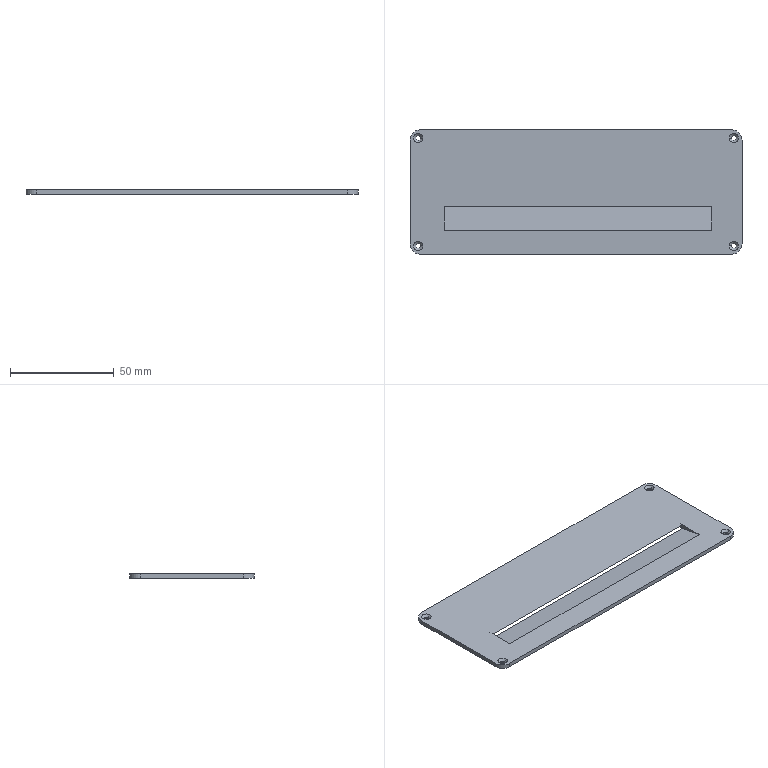Part | SolidWorks | features ICE 2, Extrusion 1, Fillet 1, HoleWzd 1 | 1 solid | 30 faces | box 160 x 60 x 2 mm | volume 16130 mm3 | cylinder 12 | plane 10 | cone 8 | commonest cylinder face diameters 2.4 x8 10 x4
STEP:
#1=CARTESIAN_POINT('',(-77.2,26.,0.95));
#2=VERTEX_POINT('',#1);
#3=CARTESIAN_POINT('',(-74.8,26.,0.95));
#4=VERTEX_POINT('',#3);
#5=CARTESIAN_POINT('',(-76.,26.,0.95));
#6=DIRECTION('',(0.,0.,1.));
#7=DIRECTION('',(1.,0.,0.));
#8=AXIS2_PLACEMENT_3D('',#5,#6,#7);
#9=CIRCLE('',#8,1.2);
#10=EDGE_CURVE('',#2,#4,#9,.T.);
#11=ORIENTED_EDGE('',*,*,#10,.F.);
#12=CARTESIAN_POINT('',(-78.25,26.,2.));
#13=VERTEX_POINT('',#12);
#14=CARTESIAN_POINT('',(-78.25,26.,2.));
#15=DIRECTION('',(-0.7071,0.,0.7071));
#16=VECTOR('',#15,1000.);
#17=LINE('',#14,#16);
#18=EDGE_CURVE('',#2,#13,#17,.T.);
#19=ORIENTED_EDGE('',*,*,#18,.T.);
#20=CARTESIAN_POINT('',(-73.75,26.,2.));
#21=VERTEX_POINT('',#20);
#22=CARTESIAN_POINT('',(-76.,26.,2.));
#23=DIRECTION('',(0.,0.,1.));
#24=DIRECTION('',(1.,0.,0.));
#25=AXIS2_PLACEMENT_3D('',#22,#23,#24);
#26=CIRCLE('',#25,2.25);
#27=EDGE_CURVE('',#13,#21,#26,.T.);
#28=ORIENTED_EDGE('',*,*,#27,.T.);
#29=CARTESIAN_POINT('',(-73.75,26.,2.));
#30=DIRECTION('',(0.7071,0.,0.7071));
#31=VECTOR('',#30,1000.);
#32=LINE('',#29,#31);
#33=EDGE_CURVE('',#4,#21,#32,.T.);
#34=ORIENTED_EDGE('',*,*,#33,.F.);
#35=EDGE_LOOP('',(#11,#19,#28,#34));
#36=FACE_OUTER_BOUND('',#35,.T.);
#37=CARTESIAN_POINT('',(-76.,26.,2.));
#38=DIRECTION('',(0.,0.,1.));
#39=DIRECTION('',(1.,0.,0.));
#40=AXIS2_PLACEMENT_3D('',#37,#38,#39);
#41=CONICAL_SURFACE('',#40,2.25,0.7854);
#42=ADVANCED_FACE('',(#36),#41,.F.);
#43=CARTESIAN_POINT('',(-74.8,26.,0.));
#44=VERTEX_POINT('',#43);
#45=CARTESIAN_POINT('',(-77.2,26.,0.));
#46=VERTEX_POINT('',#45);
#47=CARTESIAN_POINT('',(-76.,26.,0.));
#48=DIRECTION('',(0.,0.,-1.));
#49=DIRECTION('',(-1.,0.,0.));
#50=AXIS2_PLACEMENT_3D('',#47,#48,#49);
#51=CIRCLE('',#50,1.2);
#52=EDGE_CURVE('',#44,#46,#51,.T.);
#53=ORIENTED_EDGE('',*,*,#52,.T.);
#54=CARTESIAN_POINT('',(-77.2,26.,2.));
#55=DIRECTION('',(0.,0.,1.));
#56=VECTOR('',#55,1000.);
#57=LINE('',#54,#56);
#58=EDGE_CURVE('',#46,#2,#57,.T.);
#59=ORIENTED_EDGE('',*,*,#58,.T.);
#60=ORIENTED_EDGE('',*,*,#10,.T.);
#61=CARTESIAN_POINT('',(-74.8,26.,2.));
#62=DIRECTION('',(0.,0.,1.));
#63=VECTOR('',#62,1000.);
#64=LINE('',#61,#63);
#65=EDGE_CURVE('',#44,#4,#64,.T.);
#66=ORIENTED_EDGE('',*,*,#65,.F.);
#67=EDGE_LOOP('',(#53,#59,#60,#66));
#68=FACE_OUTER_BOUND('',#67,.T.);
#69=CARTESIAN_POINT('',(-76.,26.,2.));
#70=DIRECTION('',(0.,0.,1.));
#71=DIRECTION('',(1.,0.,0.));
#72=AXIS2_PLACEMENT_3D('',#69,#70,#71);
#73=CYLINDRICAL_SURFACE('',#72,1.2);
#74=ADVANCED_FACE('',(#68),#73,.F.);
#75=CARTESIAN_POINT('',(74.8,26.,0.95));
#76=VERTEX_POINT('',#75);
#77=CARTESIAN_POINT('',(77.2,26.,0.95));
#78=VERTEX_POINT('',#77);
#79=CARTESIAN_POINT('',(76.,26.,0.95));
#80=DIRECTION('',(0.,0.,1.));
#81=DIRECTION('',(1.,0.,0.));
#82=AXIS2_PLACEMENT_3D('',#79,#80,#81);
#83=CIRCLE('',#82,1.2);
#84=EDGE_CURVE('',#76,#78,#83,.T.);
#85=ORIENTED_EDGE('',*,*,#84,.F.);
#86=CARTESIAN_POINT('',(73.75,26.,2.));
#87=VERTEX_POINT('',#86);
#88=CARTESIAN_POINT('',(73.75,26.,2.));
#89=DIRECTION('',(-0.7071,0.,0.7071));
#90=VECTOR('',#89,1000.);
#91=LINE('',#88,#90);
#92=EDGE_CURVE('',#76,#87,#91,.T.);
#93=ORIENTED_EDGE('',*,*,#92,.T.);
#94=CARTESIAN_POINT('',(78.25,26.,2.));
#95=VERTEX_POINT('',#94);
#96=CARTESIAN_POINT('',(76.,26.,2.));
#97=DIRECTION('',(0.,0.,1.));
#98=DIRECTION('',(1.,0.,0.));
#99=AXIS2_PLACEMENT_3D('',#96,#97,#98);
#100=CIRCLE('',#99,2.25);
#101=EDGE_CURVE('',#87,#95,#100,.T.);
#102=ORIENTED_EDGE('',*,*,#101,.T.);
#103=CARTESIAN_POINT('',(78.25,26.,2.));
#104=DIRECTION('',(0.7071,0.,0.7071));
#105=VECTOR('',#104,1000.);
#106=LINE('',#103,#105);
#107=EDGE_CURVE('',#78,#95,#106,.T.);
#108=ORIENTED_EDGE('',*,*,#107,.F.);
#109=EDGE_LOOP('',(#85,#93,#102,#108));
#110=FACE_OUTER_BOUND('',#109,.T.);
#111=CARTESIAN_POINT('',(76.,26.,2.));
#112=DIRECTION('',(0.,0.,1.));
#113=DIRECTION('',(1.,0.,0.));
#114=AXIS2_PLACEMENT_3D('',#111,#112,#113);
#115=CONICAL_SURFACE('',#114,2.25,0.7854);
#116=ADVANCED_FACE('',(#110),#115,.F.);
#117=CARTESIAN_POINT('',(77.2,26.,0.));
#118=VERTEX_POINT('',#117);
#119=CARTESIAN_POINT('',(74.8,26.,0.));
#120=VERTEX_POINT('',#119);
#121=CARTESIAN_POINT('',(76.,26.,0.));
#122=DIRECTION('',(0.,0.,-1.));
#123=DIRECTION('',(-1.,0.,0.));
#124=AXIS2_PLACEMENT_3D('',#121,#122,#123);
#125=CIRCLE('',#124,1.2);
#126=EDGE_CURVE('',#118,#120,#125,.T.);
#127=ORIENTED_EDGE('',*,*,#126,.T.);
#128=CARTESIAN_POINT('',(74.8,26.,2.));
#129=DIRECTION('',(0.,0.,1.));
#130=VECTOR('',#129,1000.);
#131=LINE('',#128,#130);
#132=EDGE_CURVE('',#120,#76,#131,.T.);
#133=ORIENTED_EDGE('',*,*,#132,.T.);
#134=ORIENTED_EDGE('',*,*,#84,.T.);
#135=CARTESIAN_POINT('',(77.2,26.,2.));
#136=DIRECTION('',(0.,0.,1.));
#137=VECTOR('',#136,1000.);
#138=LINE('',#135,#137);
#139=EDGE_CURVE('',#118,#78,#138,.T.);
#140=ORIENTED_EDGE('',*,*,#139,.F.);
#141=EDGE_LOOP('',(#127,#133,#134,#140));
#142=FACE_OUTER_BOUND('',#141,.T.);
#143=CARTESIAN_POINT('',(76.,26.,2.));
#144=DIRECTION('',(0.,0.,1.));
#145=DIRECTION('',(1.,0.,0.));
#146=AXIS2_PLACEMENT_3D('',#143,#144,#145);
#147=CYLINDRICAL_SURFACE('',#146,1.2);
#148=ADVANCED_FACE('',(#142),#147,.F.);
#149=CARTESIAN_POINT('',(74.8,-26.,0.95));
#150=VERTEX_POINT('',#149);
#151=CARTESIAN_POINT('',(77.2,-26.,0.95));
#152=VERTEX_POINT('',#151);
#153=CARTESIAN_POINT('',(76.,-26.,0.95));
#154=DIRECTION('',(0.,0.,1.));
#155=DIRECTION('',(1.,0.,0.));
#156=AXIS2_PLACEMENT_3D('',#153,#154,#155);
#157=CIRCLE('',#156,1.2);
#158=EDGE_CURVE('',#150,#152,#157,.T.);
#159=ORIENTED_EDGE('',*,*,#158,.F.);
#160=CARTESIAN_POINT('',(73.75,-26.,2.));
#161=VERTEX_POINT('',#160);
#162=CARTESIAN_POINT('',(73.75,-26.,2.));
#163=DIRECTION('',(-0.7071,0.,0.7071));
#164=VECTOR('',#163,1000.);
#165=LINE('',#162,#164);
#166=EDGE_CURVE('',#150,#161,#165,.T.);
#167=ORIENTED_EDGE('',*,*,#166,.T.);
#168=CARTESIAN_POINT('',(78.25,-26.,2.));
#169=VERTEX_POINT('',#168);
#170=CARTESIAN_POINT('',(76.,-26.,2.));
#171=DIRECTION('',(0.,0.,1.));
#172=DIRECTION('',(1.,0.,0.));
#173=AXIS2_PLACEMENT_3D('',#170,#171,#172);
#174=CIRCLE('',#173,2.25);
#175=EDGE_CURVE('',#161,#169,#174,.T.);
#176=ORIENTED_EDGE('',*,*,#175,.T.);
#177=CARTESIAN_POINT('',(78.25,-26.,2.));
#178=DIRECTION('',(0.7071,0.,0.7071));
#179=VECTOR('',#178,1000.);
#180=LINE('',#177,#179);
#181=EDGE_CURVE('',#152,#169,#180,.T.);
#182=ORIENTED_EDGE('',*,*,#181,.F.);
#183=EDGE_LOOP('',(#159,#167,#176,#182));
#184=FACE_OUTER_BOUND('',#183,.T.);
#185=CARTESIAN_POINT('',(76.,-26.,2.));
#186=DIRECTION('',(0.,0.,1.));
#187=DIRECTION('',(1.,0.,0.));
#188=AXIS2_PLACEMENT_3D('',#185,#186,#187);
#189=CONICAL_SURFACE('',#188,2.25,0.7854);
#190=ADVANCED_FACE('',(#184),#189,.F.);
#191=CARTESIAN_POINT('',(77.2,-26.,0.));
#192=VERTEX_POINT('',#191);
#193=CARTESIAN_POINT('',(74.8,-26.,0.));
#194=VERTEX_POINT('',#193);
#195=CARTESIAN_POINT('',(76.,-26.,0.));
#196=DIRECTION('',(0.,0.,-1.));
#197=DIRECTION('',(-1.,0.,0.));
#198=AXIS2_PLACEMENT_3D('',#195,#196,#197);
#199=CIRCLE('',#198,1.2);
#200=EDGE_CURVE('',#192,#194,#199,.T.);
#201=ORIENTED_EDGE('',*,*,#200,.T.);
#202=CARTESIAN_POINT('',(74.8,-26.,2.));
#203=DIRECTION('',(0.,0.,1.));
#204=VECTOR('',#203,1000.);
#205=LINE('',#202,#204);
#206=EDGE_CURVE('',#194,#150,#205,.T.);
#207=ORIENTED_EDGE('',*,*,#206,.T.);
#208=ORIENTED_EDGE('',*,*,#158,.T.);
#209=CARTESIAN_POINT('',(77.2,-26.,2.));
#210=DIRECTION('',(0.,0.,1.));
#211=VECTOR('',#210,1000.);
#212=LINE('',#209,#211);
#213=EDGE_CURVE('',#192,#152,#212,.T.);
#214=ORIENTED_EDGE('',*,*,#213,.F.);
#215=EDGE_LOOP('',(#201,#207,#208,#214));
#216=FACE_OUTER_BOUND('',#215,.T.);
#217=CARTESIAN_POINT('',(76.,-26.,2.));
#218=DIRECTION('',(0.,0.,1.));
#219=DIRECTION('',(1.,0.,0.));
#220=AXIS2_PLACEMENT_3D('',#217,#218,#219);
#221=CYLINDRICAL_SURFACE('',#220,1.2);
#222=ADVANCED_FACE('',(#216),#221,.F.);
#223=CARTESIAN_POINT('',(-77.2,-26.,0.95));
#224=VERTEX_POINT('',#223);
#225=CARTESIAN_POINT('',(-74.8,-26.,0.95));
#226=VERTEX_POINT('',#225);
#227=CARTESIAN_POINT('',(-76.,-26.,0.95));
#228=DIRECTION('',(0.,0.,1.));
#229=DIRECTION('',(1.,0.,0.));
#230=AXIS2_PLACEMENT_3D('',#227,#228,#229);
#231=CIRCLE('',#230,1.2);
#232=EDGE_CURVE('',#224,#226,#231,.T.);
#233=ORIENTED_EDGE('',*,*,#232,.F.);
#234=CARTESIAN_POINT('',(-78.25,-26.,2.));
#235=VERTEX_POINT('',#234);
#236=CARTESIAN_POINT('',(-78.25,-26.,2.));
#237=DIRECTION('',(-0.7071,0.,0.7071));
#238=VECTOR('',#237,1000.);
#239=LINE('',#236,#238);
#240=EDGE_CURVE('',#224,#235,#239,.T.);
#241=ORIENTED_EDGE('',*,*,#240,.T.);
#242=CARTESIAN_POINT('',(-73.75,-26.,2.));
#243=VERTEX_POINT('',#242);
#244=CARTESIAN_POINT('',(-76.,-26.,2.));
#245=DIRECTION('',(0.,0.,1.));
#246=DIRECTION('',(1.,0.,0.));
#247=AXIS2_PLACEMENT_3D('',#244,#245,#246);
#248=CIRCLE('',#247,2.25);
#249=EDGE_CURVE('',#235,#243,#248,.T.);
#250=ORIENTED_EDGE('',*,*,#249,.T.);
#251=CARTESIAN_POINT('',(-73.75,-26.,2.));
#252=DIRECTION('',(0.7071,0.,0.7071));
#253=VECTOR('',#252,1000.);
#254=LINE('',#251,#253);
#255=EDGE_CURVE('',#226,#243,#254,.T.);
#256=ORIENTED_EDGE('',*,*,#255,.F.);
#257=EDGE_LOOP('',(#233,#241,#250,#256));
#258=FACE_OUTER_BOUND('',#257,.T.);
#259=CARTESIAN_POINT('',(-76.,-26.,2.));
#260=DIRECTION('',(0.,0.,1.));
#261=DIRECTION('',(1.,0.,0.));
#262=AXIS2_PLACEMENT_3D('',#259,#260,#261);
#263=CONICAL_SURFACE('',#262,2.25,0.7854);
#264=ADVANCED_FACE('',(#258),#263,.F.);
#265=CARTESIAN_POINT('',(-74.8,-26.,0.));
#266=VERTEX_POINT('',#265);
#267=CARTESIAN_POINT('',(-77.2,-26.,0.));
#268=VERTEX_POINT('',#267);
#269=CARTESIAN_POINT('',(-76.,-26.,0.));
#270=DIRECTION('',(0.,0.,-1.));
#271=DIRECTION('',(-1.,0.,0.));
#272=AXIS2_PLACEMENT_3D('',#269,#270,#271);
#273=CIRCLE('',#272,1.2);
#274=EDGE_CURVE('',#266,#268,#273,.T.);
#275=ORIENTED_EDGE('',*,*,#274,.T.);
#276=CARTESIAN_POINT('',(-77.2,-26.,2.));
#277=DIRECTION('',(0.,0.,1.));
#278=VECTOR('',#277,1000.);
#279=LINE('',#276,#278);
#280=EDGE_CURVE('',#268,#224,#279,.T.);
#281=ORIENTED_EDGE('',*,*,#280,.T.);
#282=ORIENTED_EDGE('',*,*,#232,.T.);
#283=CARTESIAN_POINT('',(-74.8,-26.,2.));
#284=DIRECTION('',(0.,0.,1.));
#285=VECTOR('',#284,1000.);
#286=LINE('',#283,#285);
#287=EDGE_CURVE('',#266,#226,#286,.T.);
#288=ORIENTED_EDGE('',*,*,#287,.F.);
#289=EDGE_LOOP('',(#275,#281,#282,#288));
#290=FACE_OUTER_BOUND('',#289,.T.);
#291=CARTESIAN_POINT('',(-76.,-26.,2.));
#292=DIRECTION('',(0.,0.,1.));
#293=DIRECTION('',(1.,0.,0.));
#294=AXIS2_PLACEMENT_3D('',#291,#292,#293);
#295=CYLINDRICAL_SURFACE('',#294,1.2);
#296=ADVANCED_FACE('',(#290),#295,.F.);
#297=CARTESIAN_POINT('',(65.429,-18.477,2.));
#298=VERTEX_POINT('',#297);
#299=CARTESIAN_POINT('',(-63.487,-18.477,2.));
#300=VERTEX_POINT('',#299);
#301=CARTESIAN_POINT('',(0.,-18.477,2.));
#302=DIRECTION('',(-1.,0.,0.));
#303=VECTOR('',#302,1000.);
#304=LINE('',#301,#303);
#305=EDGE_CURVE('',#298,#300,#304,.T.);
#306=ORIENTED_EDGE('',*,*,#305,.T.);
#307=CARTESIAN_POINT('',(-63.487,-6.959,2.));
#308=VERTEX_POINT('',#307);
#309=CARTESIAN_POINT('',(-63.487,0.,2.));
#310=DIRECTION('',(0.,1.,0.));
#311=VECTOR('',#310,1000.);
#312=LINE('',#309,#311);
#313=EDGE_CURVE('',#300,#308,#312,.T.);
#314=ORIENTED_EDGE('',*,*,#313,.T.);
#315=CARTESIAN_POINT('',(65.429,-6.959,2.));
#316=VERTEX_POINT('',#315);
#317=CARTESIAN_POINT('',(0.,-6.959,2.));
#318=DIRECTION('',(1.,0.,0.));
#319=VECTOR('',#318,1000.);
#320=LINE('',#317,#319);
#321=EDGE_CURVE('',#308,#316,#320,.T.);
#322=ORIENTED_EDGE('',*,*,#321,.T.);
#323=CARTESIAN_POINT('',(65.429,0.,2.));
#324=DIRECTION('',(0.,-1.,0.));
#325=VECTOR('',#324,1000.);
#326=LINE('',#323,#325);
#327=EDGE_CURVE('',#316,#298,#326,.T.);
#328=ORIENTED_EDGE('',*,*,#327,.T.);
#329=EDGE_LOOP('',(#306,#314,#322,#328));
#330=FACE_BOUND('',#329,.T.);
#331=CARTESIAN_POINT('',(76.,26.,2.));
#332=DIRECTION('',(0.,0.,1.));
#333=DIRECTION('',(1.,0.,0.));
#334=AXIS2_PLACEMENT_3D('',#331,#332,#333);
#335=CIRCLE('',#334,2.25);
#336=EDGE_CURVE('',#95,#87,#335,.T.);
#337=ORIENTED_EDGE('',*,*,#336,.F.);
#338=ORIENTED_EDGE('',*,*,#101,.F.);
#339=EDGE_LOOP('',(#337,#338));
#340=FACE_BOUND('',#339,.T.);
#341=CARTESIAN_POINT('',(76.,-26.,2.));
#342=DIRECTION('',(0.,0.,1.));
#343=DIRECTION('',(1.,0.,0.));
#344=AXIS2_PLACEMENT_3D('',#341,#342,#343);
#345=CIRCLE('',#344,2.25);
#346=EDGE_CURVE('',#169,#161,#345,.T.);
#347=ORIENTED_EDGE('',*,*,#346,.F.);
#348=ORIENTED_EDGE('',*,*,#175,.F.);
#349=EDGE_LOOP('',(#347,#348));
#350=FACE_BOUND('',#349,.T.);
#351=CARTESIAN_POINT('',(-76.,-26.,2.));
#352=DIRECTION('',(0.,0.,1.));
#353=DIRECTION('',(1.,0.,0.));
#354=AXIS2_PLACEMENT_3D('',#351,#352,#353);
#355=CIRCLE('',#354,2.25);
#356=EDGE_CURVE('',#243,#235,#355,.T.);
#357=ORIENTED_EDGE('',*,*,#356,.F.);
#358=ORIENTED_EDGE('',*,*,#249,.F.);
#359=EDGE_LOOP('',(#357,#358));
#360=FACE_BOUND('',#359,.T.);
#361=CARTESIAN_POINT('',(-75.,-30.,2.));
#362=VERTEX_POINT('',#361);
#363=CARTESIAN_POINT('',(75.,-30.,2.));
#364=VERTEX_POINT('',#363);
#365=CARTESIAN_POINT('',(-80.,-30.,2.));
#366=DIRECTION('',(1.,0.,0.));
#367=VECTOR('',#366,1000.);
#368=LINE('',#365,#367);
#369=EDGE_CURVE('',#362,#364,#368,.T.);
#370=ORIENTED_EDGE('',*,*,#369,.T.);
#371=CARTESIAN_POINT('',(80.,-25.,2.));
#372=VERTEX_POINT('',#371);
#373=CARTESIAN_POINT('',(75.,-25.,2.));
#374=DIRECTION('',(0.,0.,1.));
#375=DIRECTION('',(-1.,0.,0.));
#376=AXIS2_PLACEMENT_3D('',#373,#374,#375);
#377=CIRCLE('',#376,5.);
#378=EDGE_CURVE('',#364,#372,#377,.T.);
#379=ORIENTED_EDGE('',*,*,#378,.T.);
#380=CARTESIAN_POINT('',(80.,25.,2.));
#381=VERTEX_POINT('',#380);
#382=CARTESIAN_POINT('',(80.,-30.,2.));
#383=DIRECTION('',(0.,1.,0.));
#384=VECTOR('',#383,1000.);
#385=LINE('',#382,#384);
#386=EDGE_CURVE('',#372,#381,#385,.T.);
#387=ORIENTED_EDGE('',*,*,#386,.T.);
#388=CARTESIAN_POINT('',(75.,30.,2.));
#389=VERTEX_POINT('',#388);
#390=CARTESIAN_POINT('',(75.,25.,2.));
#391=DIRECTION('',(0.,0.,1.));
#392=DIRECTION('',(-1.,0.,0.));
#393=AXIS2_PLACEMENT_3D('',#390,#391,#392);
#394=CIRCLE('',#393,5.);
#395=EDGE_CURVE('',#381,#389,#394,.T.);
#396=ORIENTED_EDGE('',*,*,#395,.T.);
#397=CARTESIAN_POINT('',(-75.,30.,2.));
#398=VERTEX_POINT('',#397);
#399=CARTESIAN_POINT('',(-80.,30.,2.));
#400=DIRECTION('',(-1.,0.,0.));
#401=VECTOR('',#400,1000.);
#402=LINE('',#399,#401);
#403=EDGE_CURVE('',#389,#398,#402,.T.);
#404=ORIENTED_EDGE('',*,*,#403,.T.);
#405=CARTESIAN_POINT('',(-80.,25.,2.));
#406=VERTEX_POINT('',#405);
#407=CARTESIAN_POINT('',(-75.,25.,2.));
#408=DIRECTION('',(0.,0.,1.));
#409=DIRECTION('',(-1.,0.,0.));
#410=AXIS2_PLACEMENT_3D('',#407,#408,#409);
#411=CIRCLE('',#410,5.);
#412=EDGE_CURVE('',#398,#406,#411,.T.);
#413=ORIENTED_EDGE('',*,*,#412,.T.);
#414=CARTESIAN_POINT('',(-80.,-25.,2.));
#415=VERTEX_POINT('',#414);
#416=CARTESIAN_POINT('',(-80.,-30.,2.));
#417=DIRECTION('',(0.,-1.,0.));
#418=VECTOR('',#417,1000.);
#419=LINE('',#416,#418);
#420=EDGE_CURVE('',#406,#415,#419,.T.);
#421=ORIENTED_EDGE('',*,*,#420,.T.);
#422=CARTESIAN_POINT('',(-75.,-25.,2.));
#423=DIRECTION('',(0.,0.,1.));
#424=DIRECTION('',(-1.,0.,0.));
#425=AXIS2_PLACEMENT_3D('',#422,#423,#424);
#426=CIRCLE('',#425,5.);
#427=EDGE_CURVE('',#415,#362,#426,.T.);
#428=ORIENTED_EDGE('',*,*,#427,.T.);
#429=EDGE_LOOP('',(#370,#379,#387,#396,#404,#413,#421,#428));
#430=FACE_OUTER_BOUND('',#429,.T.);
#431=CARTESIAN_POINT('',(-76.,26.,2.));
#432=DIRECTION('',(0.,0.,1.));
#433=DIRECTION('',(1.,0.,0.));
#434=AXIS2_PLACEMENT_3D('',#431,#432,#433);
#435=CIRCLE('',#434,2.25);
#436=EDGE_CURVE('',#21,#13,#435,.T.);
#437=ORIENTED_EDGE('',*,*,#436,.F.);
#438=ORIENTED_EDGE('',*,*,#27,.F.);
#439=EDGE_LOOP('',(#437,#438));
#440=FACE_BOUND('',#439,.T.);
#441=CARTESIAN_POINT('',(0.,0.,2.));
#442=DIRECTION('',(0.,0.,-1.));
#443=DIRECTION('',(-1.,0.,0.));
#444=AXIS2_PLACEMENT_3D('',#441,#442,#443);
#445=PLANE('',#444);
#446=ADVANCED_FACE('',(#330,#340,#350,#360,#430,#440),#445,.F.);
#447=ORIENTED_EDGE('',*,*,#386,.F.);
#448=CARTESIAN_POINT('',(80.,-25.,0.));
#449=VERTEX_POINT('',#448);
#450=CARTESIAN_POINT('',(80.,-25.,2.));
#451=DIRECTION('',(0.,0.,-1.));
#452=VECTOR('',#451,1000.);
#453=LINE('',#450,#452);
#454=EDGE_CURVE('',#372,#449,#453,.T.);
#455=ORIENTED_EDGE('',*,*,#454,.T.);
#456=CARTESIAN_POINT('',(80.,25.,0.));
#457=VERTEX_POINT('',#456);
#458=CARTESIAN_POINT('',(80.,-30.,0.));
#459=DIRECTION('',(0.,1.,0.));
#460=VECTOR('',#459,1000.);
#461=LINE('',#458,#460);
#462=EDGE_CURVE('',#449,#457,#461,.T.);
#463=ORIENTED_EDGE('',*,*,#462,.T.);
#464=CARTESIAN_POINT('',(80.,25.,2.));
#465=DIRECTION('',(0.,0.,1.));
#466=VECTOR('',#465,1000.);
#467=LINE('',#464,#466);
#468=EDGE_CURVE('',#457,#381,#467,.T.);
#469=ORIENTED_EDGE('',*,*,#468,.T.);
#470=EDGE_LOOP('',(#447,#455,#463,#469));
#471=FACE_OUTER_BOUND('',#470,.T.);
#472=CARTESIAN_POINT('',(80.,-30.,2.));
#473=DIRECTION('',(-1.,0.,0.));
#474=DIRECTION('',(0.,0.,1.));
#475=AXIS2_PLACEMENT_3D('',#472,#473,#474);
#476=PLANE('',#475);
#477=ADVANCED_FACE('',(#471),#476,.F.);
#478=ORIENTED_EDGE('',*,*,#403,.F.);
#479=CARTESIAN_POINT('',(75.,30.,0.));
#480=VERTEX_POINT('',#479);
#481=CARTESIAN_POINT('',(75.,30.,2.));
#482=DIRECTION('',(0.,0.,-1.));
#483=VECTOR('',#482,1000.);
#484=LINE('',#481,#483);
#485=EDGE_CURVE('',#389,#480,#484,.T.);
#486=ORIENTED_EDGE('',*,*,#485,.T.);
#487=CARTESIAN_POINT('',(-75.,30.,0.));
#488=VERTEX_POINT('',#487);
#489=CARTESIAN_POINT('',(-80.,30.,0.));
#490=DIRECTION('',(-1.,0.,0.));
#491=VECTOR('',#490,1000.);
#492=LINE('',#489,#491);
#493=EDGE_CURVE('',#480,#488,#492,.T.);
#494=ORIENTED_EDGE('',*,*,#493,.T.);
#495=CARTESIAN_POINT('',(-75.,30.,2.));
#496=DIRECTION('',(0.,0.,1.));
#497=VECTOR('',#496,1000.);
#498=LINE('',#495,#497);
#499=EDGE_CURVE('',#488,#398,#498,.T.);
#500=ORIENTED_EDGE('',*,*,#499,.T.);
#501=EDGE_LOOP('',(#478,#486,#494,#500));
#502=FACE_OUTER_BOUND('',#501,.T.);
#503=CARTESIAN_POINT('',(-80.,30.,2.));
#504=DIRECTION('',(0.,-1.,0.));
#505=DIRECTION('',(0.,0.,-1.));
#506=AXIS2_PLACEMENT_3D('',#503,#504,#505);
#507=PLANE('',#506);
#508=ADVANCED_FACE('',(#502),#507,.F.);
#509=CARTESIAN_POINT('',(-80.,25.,0.));
#510=VERTEX_POINT('',#509);
#511=CARTESIAN_POINT('',(-80.,-25.,0.));
#512=VERTEX_POINT('',#511);
#513=CARTESIAN_POINT('',(-80.,-30.,0.));
#514=DIRECTION('',(0.,-1.,0.));
#515=VECTOR('',#514,1000.);
#516=LINE('',#513,#515);
#517=EDGE_CURVE('',#510,#512,#516,.T.);
#518=ORIENTED_EDGE('',*,*,#517,.T.);
#519=CARTESIAN_POINT('',(-80.,-25.,2.));
#520=DIRECTION('',(0.,0.,1.));
#521=VECTOR('',#520,1000.);
#522=LINE('',#519,#521);
#523=EDGE_CURVE('',#512,#415,#522,.T.);
#524=ORIENTED_EDGE('',*,*,#523,.T.);
#525=ORIENTED_EDGE('',*,*,#420,.F.);
#526=CARTESIAN_POINT('',(-80.,25.,2.));
#527=DIRECTION('',(0.,0.,-1.));
#528=VECTOR('',#527,1000.);
#529=LINE('',#526,#528);
#530=EDGE_CURVE('',#406,#510,#529,.T.);
#531=ORIENTED_EDGE('',*,*,#530,.T.);
#532=EDGE_LOOP('',(#518,#524,#525,#531));
#533=FACE_OUTER_BOUND('',#532,.T.);
#534=CARTESIAN_POINT('',(-80.,-30.,2.));
#535=DIRECTION('',(1.,0.,0.));
#536=DIRECTION('',(0.,0.,-1.));
#537=AXIS2_PLACEMENT_3D('',#534,#535,#536);
#538=PLANE('',#537);
#539=ADVANCED_FACE('',(#533),#538,.F.);
#540=CARTESIAN_POINT('',(-75.,-30.,0.));
#541=VERTEX_POINT('',#540);
#542=CARTESIAN_POINT('',(75.,-30.,0.));
#543=VERTEX_POINT('',#542);
#544=CARTESIAN_POINT('',(-80.,-30.,0.));
#545=DIRECTION('',(1.,0.,0.));
#546=VECTOR('',#545,1000.);
#547=LINE('',#544,#546);
#548=EDGE_CURVE('',#541,#543,#547,.T.);
#549=ORIENTED_EDGE('',*,*,#548,.T.);
#550=CARTESIAN_POINT('',(75.,-30.,2.));
#551=DIRECTION('',(0.,0.,1.));
#552=VECTOR('',#551,1000.);
#553=LINE('',#550,#552);
#554=EDGE_CURVE('',#543,#364,#553,.T.);
#555=ORIENTED_EDGE('',*,*,#554,.T.);
#556=ORIENTED_EDGE('',*,*,#369,.F.);
#557=CARTESIAN_POINT('',(-75.,-30.,2.));
#558=DIRECTION('',(0.,0.,-1.));
#559=VECTOR('',#558,1000.);
#560=LINE('',#557,#559);
#561=EDGE_CURVE('',#362,#541,#560,.T.);
#562=ORIENTED_EDGE('',*,*,#561,.T.);
#563=EDGE_LOOP('',(#549,#555,#556,#562));
#564=FACE_OUTER_BOUND('',#563,.T.);
#565=CARTESIAN_POINT('',(-80.,-30.,2.));
#566=DIRECTION('',(0.,1.,0.));
#567=DIRECTION('',(0.,0.,1.));
#568=AXIS2_PLACEMENT_3D('',#565,#566,#567);
#569=PLANE('',#568);
#570=ADVANCED_FACE('',(#564),#569,.F.);
#571=CARTESIAN_POINT('',(-63.487,-7.134,0.));
#572=VERTEX_POINT('',#571);
#573=CARTESIAN_POINT('',(-63.487,4.383,0.));
#574=VERTEX_POINT('',#573);
#575=CARTESIAN_POINT('',(-63.487,0.,0.));
#576=DIRECTION('',(0.,1.,0.));
#577=VECTOR('',#576,1000.);
#578=LINE('',#575,#577);
#579=EDGE_CURVE('',#572,#574,#578,.T.);
#580=ORIENTED_EDGE('',*,*,#579,.F.);
#581=CARTESIAN_POINT('',(65.429,-7.134,0.));
#582=VERTEX_POINT('',#581);
#583=CARTESIAN_POINT('',(0.,-7.134,0.));
#584=DIRECTION('',(-1.,0.,0.));
#585=VECTOR('',#584,1000.);
#586=LINE('',#583,#585);
#587=EDGE_CURVE('',#582,#572,#586,.T.);
#588=ORIENTED_EDGE('',*,*,#587,.F.);
#589=CARTESIAN_POINT('',(65.429,4.383,0.));
#590=VERTEX_POINT('',#589);
#591=CARTESIAN_POINT('',(65.429,0.,0.));
#592=DIRECTION('',(0.,-1.,0.));
#593=VECTOR('',#592,1000.);
#594=LINE('',#591,#593);
#595=EDGE_CURVE('',#590,#582,#594,.T.);
#596=ORIENTED_EDGE('',*,*,#595,.F.);
#597=CARTESIAN_POINT('',(0.,4.383,0.));
#598=DIRECTION('',(1.,0.,0.));
#599=VECTOR('',#598,1000.);
#600=LINE('',#597,#599);
#601=EDGE_CURVE('',#574,#590,#600,.T.);
#602=ORIENTED_EDGE('',*,*,#601,.F.);
#603=EDGE_LOOP('',(#580,#588,#596,#602));
#604=FACE_BOUND('',#603,.T.);
#605=ORIENTED_EDGE('',*,*,#52,.F.);
#606=CARTESIAN_POINT('',(-76.,26.,0.));
#607=DIRECTION('',(0.,0.,-1.));
#608=DIRECTION('',(-1.,0.,0.));
#609=AXIS2_PLACEMENT_3D('',#606,#607,#608);
#610=CIRCLE('',#609,1.2);
#611=EDGE_CURVE('',#46,#44,#610,.T.);
#612=ORIENTED_EDGE('',*,*,#611,.F.);
#613=EDGE_LOOP('',(#605,#612));
#614=FACE_BOUND('',#613,.T.);
#615=ORIENTED_EDGE('',*,*,#126,.F.);
#616=CARTESIAN_POINT('',(76.,26.,0.));
#617=DIRECTION('',(0.,0.,-1.));
#618=DIRECTION('',(-1.,0.,0.));
#619=AXIS2_PLACEMENT_3D('',#616,#617,#618);
#620=CIRCLE('',#619,1.2);
#621=EDGE_CURVE('',#120,#118,#620,.T.);
#622=ORIENTED_EDGE('',*,*,#621,.F.);
#623=EDGE_LOOP('',(#615,#622));
#624=FACE_BOUND('',#623,.T.);
#625=ORIENTED_EDGE('',*,*,#200,.F.);
#626=CARTESIAN_POINT('',(76.,-26.,0.));
#627=DIRECTION('',(0.,0.,-1.));
#628=DIRECTION('',(-1.,0.,0.));
#629=AXIS2_PLACEMENT_3D('',#626,#627,#628);
#630=CIRCLE('',#629,1.2);
#631=EDGE_CURVE('',#194,#192,#630,.T.);
#632=ORIENTED_EDGE('',*,*,#631,.F.);
#633=EDGE_LOOP('',(#625,#632));
#634=FACE_BOUND('',#633,.T.);
#635=ORIENTED_EDGE('',*,*,#274,.F.);
#636=CARTESIAN_POINT('',(-76.,-26.,0.));
#637=DIRECTION('',(0.,0.,-1.));
#638=DIRECTION('',(-1.,0.,0.));
#639=AXIS2_PLACEMENT_3D('',#636,#637,#638);
#640=CIRCLE('',#639,1.2);
#641=EDGE_CURVE('',#268,#266,#640,.T.);
#642=ORIENTED_EDGE('',*,*,#641,.F.);
#643=EDGE_LOOP('',(#635,#642));
#644=FACE_BOUND('',#643,.T.);
#645=ORIENTED_EDGE('',*,*,#462,.F.);
#646=CARTESIAN_POINT('',(75.,-25.,0.));
#647=DIRECTION('',(0.,0.,-1.));
#648=DIRECTION('',(-1.,0.,0.));
#649=AXIS2_PLACEMENT_3D('',#646,#647,#648);
#650=CIRCLE('',#649,5.);
#651=EDGE_CURVE('',#449,#543,#650,.T.);
#652=ORIENTED_EDGE('',*,*,#651,.T.);
#653=ORIENTED_EDGE('',*,*,#548,.F.);
#654=CARTESIAN_POINT('',(-75.,-25.,0.));
#655=DIRECTION('',(0.,0.,-1.));
#656=DIRECTION('',(-1.,0.,0.));
#657=AXIS2_PLACEMENT_3D('',#654,#655,#656);
#658=CIRCLE('',#657,5.);
#659=EDGE_CURVE('',#541,#512,#658,.T.);
#660=ORIENTED_EDGE('',*,*,#659,.T.);
#661=ORIENTED_EDGE('',*,*,#517,.F.);
#662=CARTESIAN_POINT('',(-75.,25.,0.));
#663=DIRECTION('',(0.,0.,-1.));
#664=DIRECTION('',(-1.,0.,0.));
#665=AXIS2_PLACEMENT_3D('',#662,#663,#664);
#666=CIRCLE('',#665,5.);
#667=EDGE_CURVE('',#510,#488,#666,.T.);
#668=ORIENTED_EDGE('',*,*,#667,.T.);
#669=ORIENTED_EDGE('',*,*,#493,.F.);
#670=CARTESIAN_POINT('',(75.,25.,0.));
#671=DIRECTION('',(0.,0.,-1.));
#672=DIRECTION('',(-1.,0.,0.));
#673=AXIS2_PLACEMENT_3D('',#670,#671,#672);
#674=CIRCLE('',#673,5.);
#675=EDGE_CURVE('',#480,#457,#674,.T.);
#676=ORIENTED_EDGE('',*,*,#675,.T.);
#677=EDGE_LOOP('',(#645,#652,#653,#660,#661,#668,#669,#676));
#678=FACE_OUTER_BOUND('',#677,.T.);
#679=CARTESIAN_POINT('',(0.,0.,0.));
#680=DIRECTION('',(0.,0.,-1.));
#681=DIRECTION('',(-1.,0.,0.));
#682=AXIS2_PLACEMENT_3D('',#679,#680,#681);
#683=PLANE('',#682);
#684=ADVANCED_FACE('',(#604,#614,#624,#634,#644,#678),#683,.T.);
#685=ORIENTED_EDGE('',*,*,#280,.F.);
#686=ORIENTED_EDGE('',*,*,#641,.T.);
#687=ORIENTED_EDGE('',*,*,#287,.T.);
#688=CARTESIAN_POINT('',(-76.,-26.,0.95));
#689=DIRECTION('',(0.,0.,1.));
#690=DIRECTION('',(1.,0.,0.));
#691=AXIS2_PLACEMENT_3D('',#688,#689,#690);
#692=CIRCLE('',#691,1.2);
#693=EDGE_CURVE('',#226,#224,#692,.T.);
#694=ORIENTED_EDGE('',*,*,#693,.T.);
#695=EDGE_LOOP('',(#685,#686,#687,#694));
#696=FACE_OUTER_BOUND('',#695,.T.);
#697=CARTESIAN_POINT('',(-76.,-26.,2.));
#698=DIRECTION('',(0.,0.,1.));
#699=DIRECTION('',(1.,0.,0.));
#700=AXIS2_PLACEMENT_3D('',#697,#698,#699);
#701=CYLINDRICAL_SURFACE('',#700,1.2);
#702=ADVANCED_FACE('',(#696),#701,.F.);
#703=ORIENTED_EDGE('',*,*,#240,.F.);
#704=ORIENTED_EDGE('',*,*,#693,.F.);
#705=ORIENTED_EDGE('',*,*,#255,.T.);
#706=ORIENTED_EDGE('',*,*,#356,.T.);
#707=EDGE_LOOP('',(#703,#704,#705,#706));
#708=FACE_OUTER_BOUND('',#707,.T.);
#709=CARTESIAN_POINT('',(-76.,-26.,2.));
#710=DIRECTION('',(0.,0.,1.));
#711=DIRECTION('',(1.,0.,0.));
#712=AXIS2_PLACEMENT_3D('',#709,#710,#711);
#713=CONICAL_SURFACE('',#712,2.25,0.7854);
#714=ADVANCED_FACE('',(#708),#713,.F.);
#715=ORIENTED_EDGE('',*,*,#206,.F.);
#716=ORIENTED_EDGE('',*,*,#631,.T.);
#717=ORIENTED_EDGE('',*,*,#213,.T.);
#718=CARTESIAN_POINT('',(76.,-26.,0.95));
#719=DIRECTION('',(0.,0.,1.));
#720=DIRECTION('',(1.,0.,0.));
#721=AXIS2_PLACEMENT_3D('',#718,#719,#720);
#722=CIRCLE('',#721,1.2);
#723=EDGE_CURVE('',#152,#150,#722,.T.);
#724=ORIENTED_EDGE('',*,*,#723,.T.);
#725=EDGE_LOOP('',(#715,#716,#717,#724));
#726=FACE_OUTER_BOUND('',#725,.T.);
#727=CARTESIAN_POINT('',(76.,-26.,2.));
#728=DIRECTION('',(0.,0.,1.));
#729=DIRECTION('',(1.,0.,0.));
#730=AXIS2_PLACEMENT_3D('',#727,#728,#729);
#731=CYLINDRICAL_SURFACE('',#730,1.2);
#732=ADVANCED_FACE('',(#726),#731,.F.);
#733=ORIENTED_EDGE('',*,*,#166,.F.);
#734=ORIENTED_EDGE('',*,*,#723,.F.);
#735=ORIENTED_EDGE('',*,*,#181,.T.);
#736=ORIENTED_EDGE('',*,*,#346,.T.);
#737=EDGE_LOOP('',(#733,#734,#735,#736));
#738=FACE_OUTER_BOUND('',#737,.T.);
#739=CARTESIAN_POINT('',(76.,-26.,2.));
#740=DIRECTION('',(0.,0.,1.));
#741=DIRECTION('',(1.,0.,0.));
#742=AXIS2_PLACEMENT_3D('',#739,#740,#741);
#743=CONICAL_SURFACE('',#742,2.25,0.7854);
#744=ADVANCED_FACE('',(#738),#743,.F.);
#745=ORIENTED_EDGE('',*,*,#132,.F.);
#746=ORIENTED_EDGE('',*,*,#621,.T.);
#747=ORIENTED_EDGE('',*,*,#139,.T.);
#748=CARTESIAN_POINT('',(76.,26.,0.95));
#749=DIRECTION('',(0.,0.,1.));
#750=DIRECTION('',(1.,0.,0.));
#751=AXIS2_PLACEMENT_3D('',#748,#749,#750);
#752=CIRCLE('',#751,1.2);
#753=EDGE_CURVE('',#78,#76,#752,.T.);
#754=ORIENTED_EDGE('',*,*,#753,.T.);
#755=EDGE_LOOP('',(#745,#746,#747,#754));
#756=FACE_OUTER_BOUND('',#755,.T.);
#757=CARTESIAN_POINT('',(76.,26.,2.));
#758=DIRECTION('',(0.,0.,1.));
#759=DIRECTION('',(1.,0.,0.));
#760=AXIS2_PLACEMENT_3D('',#757,#758,#759);
#761=CYLINDRICAL_SURFACE('',#760,1.2);
#762=ADVANCED_FACE('',(#756),#761,.F.);
#763=ORIENTED_EDGE('',*,*,#92,.F.);
#764=ORIENTED_EDGE('',*,*,#753,.F.);
#765=ORIENTED_EDGE('',*,*,#107,.T.);
#766=ORIENTED_EDGE('',*,*,#336,.T.);
#767=EDGE_LOOP('',(#763,#764,#765,#766));
#768=FACE_OUTER_BOUND('',#767,.T.);
#769=CARTESIAN_POINT('',(76.,26.,2.));
#770=DIRECTION('',(0.,0.,1.));
#771=DIRECTION('',(1.,0.,0.));
#772=AXIS2_PLACEMENT_3D('',#769,#770,#771);
#773=CONICAL_SURFACE('',#772,2.25,0.7854);
#774=ADVANCED_FACE('',(#768),#773,.F.);
#775=ORIENTED_EDGE('',*,*,#58,.F.);
#776=ORIENTED_EDGE('',*,*,#611,.T.);
#777=ORIENTED_EDGE('',*,*,#65,.T.);
#778=CARTESIAN_POINT('',(-76.,26.,0.95));
#779=DIRECTION('',(0.,0.,1.));
#780=DIRECTION('',(1.,0.,0.));
#781=AXIS2_PLACEMENT_3D('',#778,#779,#780);
#782=CIRCLE('',#781,1.2);
#783=EDGE_CURVE('',#4,#2,#782,.T.);
#784=ORIENTED_EDGE('',*,*,#783,.T.);
#785=EDGE_LOOP('',(#775,#776,#777,#784));
#786=FACE_OUTER_BOUND('',#785,.T.);
#787=CARTESIAN_POINT('',(-76.,26.,2.));
#788=DIRECTION('',(0.,0.,1.));
#789=DIRECTION('',(1.,0.,0.));
#790=AXIS2_PLACEMENT_3D('',#787,#788,#789);
#791=CYLINDRICAL_SURFACE('',#790,1.2);
#792=ADVANCED_FACE('',(#786),#791,.F.);
#793=ORIENTED_EDGE('',*,*,#18,.F.);
#794=ORIENTED_EDGE('',*,*,#783,.F.);
#795=ORIENTED_EDGE('',*,*,#33,.T.);
#796=ORIENTED_EDGE('',*,*,#436,.T.);
#797=EDGE_LOOP('',(#793,#794,#795,#796));
#798=FACE_OUTER_BOUND('',#797,.T.);
#799=CARTESIAN_POINT('',(-76.,26.,2.));
#800=DIRECTION('',(0.,0.,1.));
#801=DIRECTION('',(1.,0.,0.));
#802=AXIS2_PLACEMENT_3D('',#799,#800,#801);
#803=CONICAL_SURFACE('',#802,2.25,0.7854);
#804=ADVANCED_FACE('',(#798),#803,.F.);
#805=CARTESIAN_POINT('',(-63.487,68.828,-13.394));
#806=DIRECTION('',(0.,-0.9848,0.1736));
#807=VECTOR('',#806,1000.);
#808=LINE('',#805,#807);
#809=EDGE_CURVE('',#572,#300,#808,.T.);
#810=ORIENTED_EDGE('',*,*,#809,.F.);
#811=ORIENTED_EDGE('',*,*,#579,.T.);
#812=CARTESIAN_POINT('',(-63.487,69.176,-11.425));
#813=DIRECTION('',(0.,-0.9848,0.1736));
#814=VECTOR('',#813,1000.);
#815=LINE('',#812,#814);
#816=EDGE_CURVE('',#574,#308,#815,.T.);
#817=ORIENTED_EDGE('',*,*,#816,.T.);
#818=ORIENTED_EDGE('',*,*,#313,.F.);
#819=EDGE_LOOP('',(#810,#811,#817,#818));
#820=FACE_OUTER_BOUND('',#819,.T.);
#821=CARTESIAN_POINT('',(-63.487,69.176,-11.425));
#822=DIRECTION('',(-1.,0.,0.));
#823=DIRECTION('',(0.,0.,1.));
#824=AXIS2_PLACEMENT_3D('',#821,#822,#823);
#825=PLANE('',#824);
#826=ADVANCED_FACE('',(#820),#825,.F.);
#827=ORIENTED_EDGE('',*,*,#816,.F.);
#828=ORIENTED_EDGE('',*,*,#601,.T.);
#829=CARTESIAN_POINT('',(65.429,69.176,-11.425));
#830=DIRECTION('',(0.,-0.9848,0.1736));
#831=VECTOR('',#830,1000.);
#832=LINE('',#829,#831);
#833=EDGE_CURVE('',#590,#316,#832,.T.);
#834=ORIENTED_EDGE('',*,*,#833,.T.);
#835=ORIENTED_EDGE('',*,*,#321,.F.);
#836=EDGE_LOOP('',(#827,#828,#834,#835));
#837=FACE_OUTER_BOUND('',#836,.T.);
#838=CARTESIAN_POINT('',(-63.487,69.176,-11.425));
#839=DIRECTION('',(0.,0.1736,0.9848));
#840=DIRECTION('',(0.,-0.9848,0.1736));
#841=AXIS2_PLACEMENT_3D('',#838,#839,#840);
#842=PLANE('',#841);
#843=ADVANCED_FACE('',(#837),#842,.F.);
#844=ORIENTED_EDGE('',*,*,#833,.F.);
#845=ORIENTED_EDGE('',*,*,#595,.T.);
#846=CARTESIAN_POINT('',(65.429,68.828,-13.394));
#847=DIRECTION('',(0.,-0.9848,0.1736));
#848=VECTOR('',#847,1000.);
#849=LINE('',#846,#848);
#850=EDGE_CURVE('',#582,#298,#849,.T.);
#851=ORIENTED_EDGE('',*,*,#850,.T.);
#852=ORIENTED_EDGE('',*,*,#327,.F.);
#853=EDGE_LOOP('',(#844,#845,#851,#852));
#854=FACE_OUTER_BOUND('',#853,.T.);
#855=CARTESIAN_POINT('',(65.429,69.176,-11.425));
#856=DIRECTION('',(1.,0.,0.));
#857=DIRECTION('',(0.,0.,-1.));
#858=AXIS2_PLACEMENT_3D('',#855,#856,#857);
#859=PLANE('',#858);
#860=ADVANCED_FACE('',(#854),#859,.F.);
#861=ORIENTED_EDGE('',*,*,#850,.F.);
#862=ORIENTED_EDGE('',*,*,#587,.T.);
#863=ORIENTED_EDGE('',*,*,#809,.T.);
#864=ORIENTED_EDGE('',*,*,#305,.F.);
#865=EDGE_LOOP('',(#861,#862,#863,#864));
#866=FACE_OUTER_BOUND('',#865,.T.);
#867=CARTESIAN_POINT('',(-63.487,68.828,-13.394));
#868=DIRECTION('',(0.,-0.1736,-0.9848));
#869=DIRECTION('',(0.,0.9848,-0.1736));
#870=AXIS2_PLACEMENT_3D('',#867,#868,#869);
#871=PLANE('',#870);
#872=ADVANCED_FACE('',(#866),#871,.F.);
#873=ORIENTED_EDGE('',*,*,#378,.F.);
#874=ORIENTED_EDGE('',*,*,#554,.F.);
#875=ORIENTED_EDGE('',*,*,#651,.F.);
#876=ORIENTED_EDGE('',*,*,#454,.F.);
#877=EDGE_LOOP('',(#873,#874,#875,#876));
#878=FACE_OUTER_BOUND('',#877,.T.);
#879=CARTESIAN_POINT('',(75.,-25.,2.));
#880=DIRECTION('',(0.,0.,-1.));
#881=DIRECTION('',(-1.,0.,0.));
#882=AXIS2_PLACEMENT_3D('',#879,#880,#881);
#883=CYLINDRICAL_SURFACE('',#882,5.);
#884=ADVANCED_FACE('',(#878),#883,.T.);
#885=ORIENTED_EDGE('',*,*,#427,.F.);
#886=ORIENTED_EDGE('',*,*,#523,.F.);
#887=ORIENTED_EDGE('',*,*,#659,.F.);
#888=ORIENTED_EDGE('',*,*,#561,.F.);
#889=EDGE_LOOP('',(#885,#886,#887,#888));
#890=FACE_OUTER_BOUND('',#889,.T.);
#891=CARTESIAN_POINT('',(-75.,-25.,2.));
#892=DIRECTION('',(0.,0.,-1.));
#893=DIRECTION('',(-1.,0.,0.));
#894=AXIS2_PLACEMENT_3D('',#891,#892,#893);
#895=CYLINDRICAL_SURFACE('',#894,5.);
#896=ADVANCED_FACE('',(#890),#895,.T.);
#897=ORIENTED_EDGE('',*,*,#395,.F.);
#898=ORIENTED_EDGE('',*,*,#468,.F.);
#899=ORIENTED_EDGE('',*,*,#675,.F.);
#900=ORIENTED_EDGE('',*,*,#485,.F.);
#901=EDGE_LOOP('',(#897,#898,#899,#900));
#902=FACE_OUTER_BOUND('',#901,.T.);
#903=CARTESIAN_POINT('',(75.,25.,2.));
#904=DIRECTION('',(0.,0.,-1.));
#905=DIRECTION('',(-1.,0.,0.));
#906=AXIS2_PLACEMENT_3D('',#903,#904,#905);
#907=CYLINDRICAL_SURFACE('',#906,5.);
#908=ADVANCED_FACE('',(#902),#907,.T.);
#909=ORIENTED_EDGE('',*,*,#412,.F.);
#910=ORIENTED_EDGE('',*,*,#499,.F.);
#911=ORIENTED_EDGE('',*,*,#667,.F.);
#912=ORIENTED_EDGE('',*,*,#530,.F.);
#913=EDGE_LOOP('',(#909,#910,#911,#912));
#914=FACE_OUTER_BOUND('',#913,.T.);
#915=CARTESIAN_POINT('',(-75.,25.,2.));
#916=DIRECTION('',(0.,0.,-1.));
#917=DIRECTION('',(-1.,0.,0.));
#918=AXIS2_PLACEMENT_3D('',#915,#916,#917);
#919=CYLINDRICAL_SURFACE('',#918,5.);
#920=ADVANCED_FACE('',(#914),#919,.T.);
#921=CLOSED_SHELL('',(#42,#74,#116,#148,#190,#222,#264,#296,#446,#477,#508,#539,#570,#684,#702,#714,#732,#744,#762,#774,#792,#804,#826,#843,#860,#872,#884,#896,#908,#920));
#922=MANIFOLD_SOLID_BREP('',#921);
#923=CARTESIAN_POINT('',(0.,0.,0.));
#924=DIRECTION('',(0.,0.,1.));
#925=DIRECTION('',(1.,0.,0.));
#926=AXIS2_PLACEMENT_3D('',#923,#924,#925);
#927=(LENGTH_UNIT()NAMED_UNIT(*)SI_UNIT(.MILLI.,.METRE.));
#928=UNCERTAINTY_MEASURE_WITH_UNIT(LENGTH_MEASURE(0.00001),#927,'','');
#929=(NAMED_UNIT(*)PLANE_ANGLE_UNIT()SI_UNIT($,.RADIAN.));
#930=(NAMED_UNIT(*)SI_UNIT($,.STERADIAN.)SOLID_ANGLE_UNIT());
#931=(GEOMETRIC_REPRESENTATION_CONTEXT(3)GLOBAL_UNCERTAINTY_ASSIGNED_CONTEXT((#928))GLOBAL_UNIT_ASSIGNED_CONTEXT((#927,#929,#930))REPRESENTATION_CONTEXT('',''));
#932=ADVANCED_BREP_SHAPE_REPRESENTATION('',(#922,#926),#931);